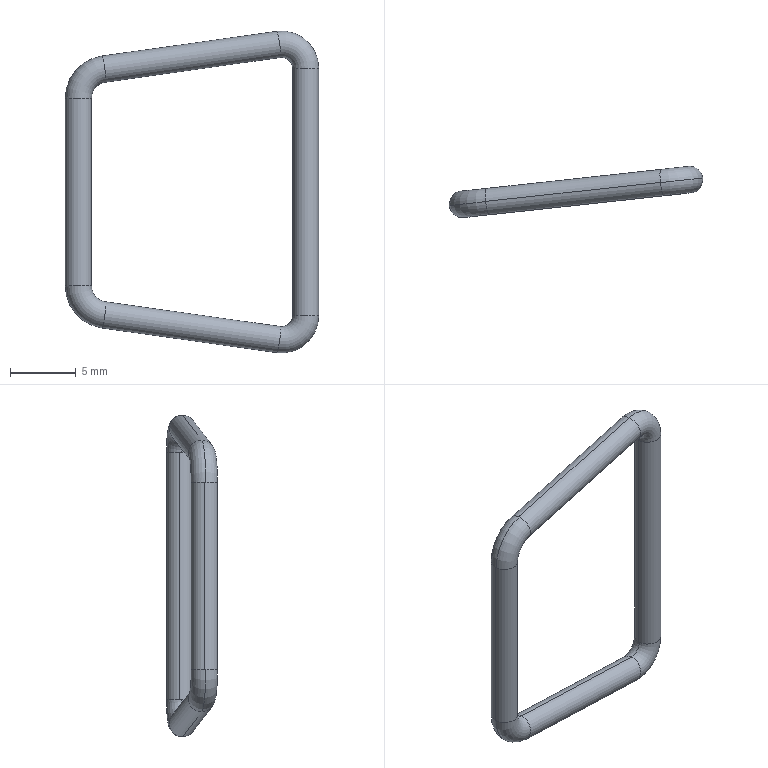Part | SolidWorks | features RefAxis 6, Revolution 4, ICE 3, 3DProfileFeature 2, Extrusion 1 | 1 solid | 16 faces | box 19.288 x 3.878 x 24.478 mm | volume 228.547 mm3 | torus 8 | cylinder 8 | commonest cylinder face diameters 2 x8
STEP:
#1=CARTESIAN_POINT('',(-18.282,-1.986,7.127));
#2=VERTEX_POINT('',#1);
#3=CARTESIAN_POINT('',(-18.288,-1.878,7.127));
#4=VERTEX_POINT('',#3);
#5=CARTESIAN_POINT('',(-17.288,-1.878,7.127));
#6=DIRECTION('',(0.,0.,-1.));
#7=DIRECTION('',(-0.9957,-0.09296,0.));
#8=AXIS2_PLACEMENT_3D('',#5,#6,#7);
#9=CIRCLE('',#8,1.);
#10=EDGE_CURVE('',#2,#4,#9,.T.);
#11=ORIENTED_EDGE('',*,*,#10,.F.);
#12=CARTESIAN_POINT('',(-15.512,-1.685,10.333));
#13=VERTEX_POINT('',#12);
#14=CARTESIAN_POINT('',(-15.064,-1.636,7.127));
#15=DIRECTION('',(-0.108,0.9942,0.));
#16=DIRECTION('',(-0.9942,-0.108,0.));
#17=AXIS2_PLACEMENT_3D('',#14,#15,#16);
#18=CIRCLE('',#17,3.237);
#19=EDGE_CURVE('',#2,#13,#18,.T.);
#20=ORIENTED_EDGE('',*,*,#19,.T.);
#21=CARTESIAN_POINT('',(-15.513,-1.67,10.333));
#22=VERTEX_POINT('',#21);
#23=CARTESIAN_POINT('',(-15.373,-1.67,9.342));
#24=DIRECTION('',(-0.9845,-0.1069,-0.1392));
#25=DIRECTION('',(-0.14,0.,0.9902));
#26=AXIS2_PLACEMENT_3D('',#23,#24,#25);
#27=CIRCLE('',#26,1.);
#28=EDGE_CURVE('',#13,#22,#27,.T.);
#29=ORIENTED_EDGE('',*,*,#28,.T.);
#30=CARTESIAN_POINT('',(-15.235,-1.655,8.352));
#31=VERTEX_POINT('',#30);
#32=CARTESIAN_POINT('',(-15.373,-1.67,9.342));
#33=DIRECTION('',(-0.9845,-0.1069,-0.1392));
#34=DIRECTION('',(-0.14,0.,0.9902));
#35=AXIS2_PLACEMENT_3D('',#32,#33,#34);
#36=CIRCLE('',#35,1.);
#37=EDGE_CURVE('',#22,#31,#36,.T.);
#38=ORIENTED_EDGE('',*,*,#37,.T.);
#39=CARTESIAN_POINT('',(-16.293,-1.77,7.127));
#40=VERTEX_POINT('',#39);
#41=CARTESIAN_POINT('',(-15.064,-1.636,7.127));
#42=DIRECTION('',(-0.108,0.9942,0.));
#43=DIRECTION('',(-0.9942,-0.108,0.));
#44=AXIS2_PLACEMENT_3D('',#41,#42,#43);
#45=CIRCLE('',#44,1.237);
#46=EDGE_CURVE('',#40,#31,#45,.T.);
#47=ORIENTED_EDGE('',*,*,#46,.F.);
#48=CARTESIAN_POINT('',(-17.288,-1.878,7.127));
#49=DIRECTION('',(0.,0.,-1.));
#50=DIRECTION('',(-0.9957,-0.09296,0.));
#51=AXIS2_PLACEMENT_3D('',#48,#49,#50);
#52=CIRCLE('',#51,1.);
#53=EDGE_CURVE('',#4,#40,#52,.T.);
#54=ORIENTED_EDGE('',*,*,#53,.F.);
#55=EDGE_LOOP('',(#11,#20,#29,#38,#47,#54));
#56=FACE_OUTER_BOUND('',#55,.T.);
#57=CARTESIAN_POINT('',(-15.064,-1.636,7.127));
#58=DIRECTION('',(-0.108,0.9942,0.));
#59=DIRECTION('',(-0.9942,-0.108,0.));
#60=AXIS2_PLACEMENT_3D('',#57,#58,#59);
#61=TOROIDAL_SURFACE('',#60,2.237,1.);
#62=ADVANCED_FACE('',(#56),#61,.T.);
#63=CARTESIAN_POINT('',(-18.282,-1.986,-7.127));
#64=VERTEX_POINT('',#63);
#65=CARTESIAN_POINT('',(-16.288,-1.878,-7.127));
#66=VERTEX_POINT('',#65);
#67=CARTESIAN_POINT('',(-17.288,-1.878,-7.127));
#68=DIRECTION('',(0.,0.,1.));
#69=DIRECTION('',(0.9957,0.09296,0.));
#70=AXIS2_PLACEMENT_3D('',#67,#68,#69);
#71=CIRCLE('',#70,1.);
#72=EDGE_CURVE('',#64,#66,#71,.T.);
#73=ORIENTED_EDGE('',*,*,#72,.F.);
#74=CARTESIAN_POINT('',(-15.512,-1.685,-10.333));
#75=VERTEX_POINT('',#74);
#76=CARTESIAN_POINT('',(-15.064,-1.636,-7.127));
#77=DIRECTION('',(0.108,-0.9942,0.));
#78=DIRECTION('',(0.9942,0.108,0.));
#79=AXIS2_PLACEMENT_3D('',#76,#77,#78);
#80=CIRCLE('',#79,3.237);
#81=EDGE_CURVE('',#64,#75,#80,.T.);
#82=ORIENTED_EDGE('',*,*,#81,.T.);
#83=CARTESIAN_POINT('',(-15.233,-1.67,-8.352));
#84=VERTEX_POINT('',#83);
#85=CARTESIAN_POINT('',(-15.373,-1.67,-9.342));
#86=DIRECTION('',(-0.9845,-0.1069,0.1392));
#87=DIRECTION('',(0.14,0.,0.9902));
#88=AXIS2_PLACEMENT_3D('',#85,#86,#87);
#89=CIRCLE('',#88,1.);
#90=EDGE_CURVE('',#75,#84,#89,.T.);
#91=ORIENTED_EDGE('',*,*,#90,.T.);
#92=CARTESIAN_POINT('',(-15.235,-1.655,-8.352));
#93=VERTEX_POINT('',#92);
#94=CARTESIAN_POINT('',(-15.373,-1.67,-9.342));
#95=DIRECTION('',(-0.9845,-0.1069,0.1392));
#96=DIRECTION('',(0.14,0.,0.9902));
#97=AXIS2_PLACEMENT_3D('',#94,#95,#96);
#98=CIRCLE('',#97,1.);
#99=EDGE_CURVE('',#84,#93,#98,.T.);
#100=ORIENTED_EDGE('',*,*,#99,.T.);
#101=CARTESIAN_POINT('',(-16.293,-1.77,-7.127));
#102=VERTEX_POINT('',#101);
#103=CARTESIAN_POINT('',(-15.064,-1.636,-7.127));
#104=DIRECTION('',(0.108,-0.9942,0.));
#105=DIRECTION('',(0.9942,0.108,0.));
#106=AXIS2_PLACEMENT_3D('',#103,#104,#105);
#107=CIRCLE('',#106,1.237);
#108=EDGE_CURVE('',#102,#93,#107,.T.);
#109=ORIENTED_EDGE('',*,*,#108,.F.);
#110=CARTESIAN_POINT('',(-17.288,-1.878,-7.127));
#111=DIRECTION('',(0.,0.,1.));
#112=DIRECTION('',(0.9957,0.09296,0.));
#113=AXIS2_PLACEMENT_3D('',#110,#111,#112);
#114=CIRCLE('',#113,1.);
#115=EDGE_CURVE('',#66,#102,#114,.T.);
#116=ORIENTED_EDGE('',*,*,#115,.F.);
#117=EDGE_LOOP('',(#73,#82,#91,#100,#109,#116));
#118=FACE_OUTER_BOUND('',#117,.T.);
#119=CARTESIAN_POINT('',(-15.064,-1.636,-7.127));
#120=DIRECTION('',(0.108,-0.9942,0.));
#121=DIRECTION('',(0.9942,0.108,0.));
#122=AXIS2_PLACEMENT_3D('',#119,#120,#121);
#123=TOROIDAL_SURFACE('',#122,2.237,1.);
#124=ADVANCED_FACE('',(#118),#123,.T.);
#125=CARTESIAN_POINT('',(-2.221,-0.2413,12.212));
#126=VERTEX_POINT('',#125);
#127=CARTESIAN_POINT('',(-2.223,-0.2263,12.211));
#128=VERTEX_POINT('',#127);
#129=CARTESIAN_POINT('',(-2.083,-0.2263,11.221));
#130=DIRECTION('',(-0.9845,-0.1069,-0.1392));
#131=DIRECTION('',(-0.1259,-0.1223,0.9845));
#132=AXIS2_PLACEMENT_3D('',#129,#130,#131);
#133=CIRCLE('',#132,1.);
#134=EDGE_CURVE('',#126,#128,#133,.T.);
#135=ORIENTED_EDGE('',*,*,#134,.F.);
#136=CARTESIAN_POINT('',(0.9942,0.108,9.4));
#137=VERTEX_POINT('',#136);
#138=CARTESIAN_POINT('',(-1.828,-0.1986,9.4));
#139=DIRECTION('',(-0.108,0.9942,0.));
#140=DIRECTION('',(-0.9942,-0.108,0.));
#141=AXIS2_PLACEMENT_3D('',#138,#139,#140);
#142=CIRCLE('',#141,2.839);
#143=EDGE_CURVE('',#126,#137,#142,.T.);
#144=ORIENTED_EDGE('',*,*,#143,.T.);
#145=CARTESIAN_POINT('',(-1.,0.,9.4));
#146=VERTEX_POINT('',#145);
#147=CARTESIAN_POINT('',(0.,0.,9.4));
#148=DIRECTION('',(0.,0.,1.));
#149=DIRECTION('',(1.,0.,0.));
#150=AXIS2_PLACEMENT_3D('',#147,#148,#149);
#151=CIRCLE('',#150,1.);
#152=EDGE_CURVE('',#137,#146,#151,.T.);
#153=ORIENTED_EDGE('',*,*,#152,.T.);
#154=CARTESIAN_POINT('',(-0.9942,-0.108,9.4));
#155=VERTEX_POINT('',#154);
#156=CARTESIAN_POINT('',(0.,0.,9.4));
#157=DIRECTION('',(0.,0.,1.));
#158=DIRECTION('',(1.,0.,0.));
#159=AXIS2_PLACEMENT_3D('',#156,#157,#158);
#160=CIRCLE('',#159,1.);
#161=EDGE_CURVE('',#146,#155,#160,.T.);
#162=ORIENTED_EDGE('',*,*,#161,.T.);
#163=CARTESIAN_POINT('',(-1.945,-0.2112,10.231));
#164=VERTEX_POINT('',#163);
#165=CARTESIAN_POINT('',(-1.828,-0.1986,9.4));
#166=DIRECTION('',(-0.108,0.9942,0.));
#167=DIRECTION('',(-0.9942,-0.108,0.));
#168=AXIS2_PLACEMENT_3D('',#165,#166,#167);
#169=CIRCLE('',#168,0.8392);
#170=EDGE_CURVE('',#164,#155,#169,.T.);
#171=ORIENTED_EDGE('',*,*,#170,.F.);
#172=CARTESIAN_POINT('',(-2.083,-0.2263,11.221));
#173=DIRECTION('',(-0.9845,-0.1069,-0.1392));
#174=DIRECTION('',(-0.1259,-0.1223,0.9845));
#175=AXIS2_PLACEMENT_3D('',#172,#173,#174);
#176=CIRCLE('',#175,1.);
#177=EDGE_CURVE('',#128,#164,#176,.T.);
#178=ORIENTED_EDGE('',*,*,#177,.F.);
#179=EDGE_LOOP('',(#135,#144,#153,#162,#171,#178));
#180=FACE_OUTER_BOUND('',#179,.T.);
#181=CARTESIAN_POINT('',(-1.828,-0.1986,9.4));
#182=DIRECTION('',(-0.108,0.9942,0.));
#183=DIRECTION('',(-0.9942,-0.108,0.));
#184=AXIS2_PLACEMENT_3D('',#181,#182,#183);
#185=TOROIDAL_SURFACE('',#184,1.839,1.);
#186=ADVANCED_FACE('',(#180),#185,.T.);
#187=CARTESIAN_POINT('',(-1.943,-0.2263,-10.231));
#188=VERTEX_POINT('',#187);
#189=CARTESIAN_POINT('',(-2.221,-0.2413,-12.212));
#190=VERTEX_POINT('',#189);
#191=CARTESIAN_POINT('',(-2.083,-0.2263,-11.221));
#192=DIRECTION('',(0.9845,0.1069,-0.1392));
#193=DIRECTION('',(-0.1259,-0.1223,-0.9845));
#194=AXIS2_PLACEMENT_3D('',#191,#192,#193);
#195=CIRCLE('',#194,1.);
#196=EDGE_CURVE('',#188,#190,#195,.T.);
#197=ORIENTED_EDGE('',*,*,#196,.T.);
#198=CARTESIAN_POINT('',(0.9942,0.108,-9.4));
#199=VERTEX_POINT('',#198);
#200=CARTESIAN_POINT('',(-1.828,-0.1986,-9.4));
#201=DIRECTION('',(0.108,-0.9942,0.));
#202=DIRECTION('',(0.9942,0.108,0.));
#203=AXIS2_PLACEMENT_3D('',#200,#201,#202);
#204=CIRCLE('',#203,2.839);
#205=EDGE_CURVE('',#190,#199,#204,.T.);
#206=ORIENTED_EDGE('',*,*,#205,.T.);
#207=CARTESIAN_POINT('',(1.,0.,-9.4));
#208=VERTEX_POINT('',#207);
#209=CARTESIAN_POINT('',(0.,0.,-9.4));
#210=DIRECTION('',(0.,0.,1.));
#211=DIRECTION('',(1.,0.,0.));
#212=AXIS2_PLACEMENT_3D('',#209,#210,#211);
#213=CIRCLE('',#212,1.);
#214=EDGE_CURVE('',#208,#199,#213,.T.);
#215=ORIENTED_EDGE('',*,*,#214,.F.);
#216=CARTESIAN_POINT('',(-0.9942,-0.108,-9.4));
#217=VERTEX_POINT('',#216);
#218=CARTESIAN_POINT('',(0.,0.,-9.4));
#219=DIRECTION('',(0.,0.,1.));
#220=DIRECTION('',(1.,0.,0.));
#221=AXIS2_PLACEMENT_3D('',#218,#219,#220);
#222=CIRCLE('',#221,1.);
#223=EDGE_CURVE('',#217,#208,#222,.T.);
#224=ORIENTED_EDGE('',*,*,#223,.F.);
#225=CARTESIAN_POINT('',(-1.945,-0.2112,-10.231));
#226=VERTEX_POINT('',#225);
#227=CARTESIAN_POINT('',(-1.828,-0.1986,-9.4));
#228=DIRECTION('',(0.108,-0.9942,0.));
#229=DIRECTION('',(0.9942,0.108,0.));
#230=AXIS2_PLACEMENT_3D('',#227,#228,#229);
#231=CIRCLE('',#230,0.8392);
#232=EDGE_CURVE('',#226,#217,#231,.T.);
#233=ORIENTED_EDGE('',*,*,#232,.F.);
#234=CARTESIAN_POINT('',(-2.083,-0.2263,-11.221));
#235=DIRECTION('',(0.9845,0.1069,-0.1392));
#236=DIRECTION('',(-0.1259,-0.1223,-0.9845));
#237=AXIS2_PLACEMENT_3D('',#234,#235,#236);
#238=CIRCLE('',#237,1.);
#239=EDGE_CURVE('',#226,#188,#238,.T.);
#240=ORIENTED_EDGE('',*,*,#239,.T.);
#241=EDGE_LOOP('',(#197,#206,#215,#224,#233,#240));
#242=FACE_OUTER_BOUND('',#241,.T.);
#243=CARTESIAN_POINT('',(-1.828,-0.1986,-9.4));
#244=DIRECTION('',(0.108,-0.9942,0.));
#245=DIRECTION('',(0.9942,0.108,0.));
#246=AXIS2_PLACEMENT_3D('',#243,#244,#245);
#247=TOROIDAL_SURFACE('',#246,1.839,1.);
#248=ADVANCED_FACE('',(#242),#247,.T.);
#249=ORIENTED_EDGE('',*,*,#53,.T.);
#250=CARTESIAN_POINT('',(-16.288,-1.878,7.127));
#251=VERTEX_POINT('',#250);
#252=CARTESIAN_POINT('',(-17.288,-1.878,7.127));
#253=DIRECTION('',(0.,0.,-1.));
#254=DIRECTION('',(-0.9957,-0.09296,0.));
#255=AXIS2_PLACEMENT_3D('',#252,#253,#254);
#256=CIRCLE('',#255,1.);
#257=EDGE_CURVE('',#40,#251,#256,.T.);
#258=ORIENTED_EDGE('',*,*,#257,.T.);
#259=CARTESIAN_POINT('',(-16.288,-1.878,7.128));
#260=DIRECTION('',(0.,0.,-1.));
#261=VECTOR('',#260,1000.);
#262=LINE('',#259,#261);
#263=EDGE_CURVE('',#251,#66,#262,.T.);
#264=ORIENTED_EDGE('',*,*,#263,.T.);
#265=ORIENTED_EDGE('',*,*,#115,.T.);
#266=CARTESIAN_POINT('',(-18.288,-1.878,-7.127));
#267=VERTEX_POINT('',#266);
#268=CARTESIAN_POINT('',(-17.288,-1.878,-7.127));
#269=DIRECTION('',(0.,0.,1.));
#270=DIRECTION('',(0.9957,0.09296,0.));
#271=AXIS2_PLACEMENT_3D('',#268,#269,#270);
#272=CIRCLE('',#271,1.);
#273=EDGE_CURVE('',#102,#267,#272,.T.);
#274=ORIENTED_EDGE('',*,*,#273,.T.);
#275=CARTESIAN_POINT('',(-18.288,-1.878,7.128));
#276=DIRECTION('',(0.,0.,-1.));
#277=VECTOR('',#276,1000.);
#278=LINE('',#275,#277);
#279=EDGE_CURVE('',#4,#267,#278,.T.);
#280=ORIENTED_EDGE('',*,*,#279,.F.);
#281=EDGE_LOOP('',(#249,#258,#264,#265,#274,#280));
#282=FACE_OUTER_BOUND('',#281,.T.);
#283=CARTESIAN_POINT('',(-17.288,-1.878,7.128));
#284=DIRECTION('',(0.,0.,-1.));
#285=DIRECTION('',(-1.,0.,0.));
#286=AXIS2_PLACEMENT_3D('',#283,#284,#285);
#287=CYLINDRICAL_SURFACE('',#286,1.);
#288=ADVANCED_FACE('',(#282),#287,.T.);
#289=ORIENTED_EDGE('',*,*,#37,.F.);
#290=CARTESIAN_POINT('',(-15.513,-1.67,10.333));
#291=DIRECTION('',(0.9845,0.1069,0.1392));
#292=VECTOR('',#291,1000.);
#293=LINE('',#290,#292);
#294=EDGE_CURVE('',#22,#128,#293,.T.);
#295=ORIENTED_EDGE('',*,*,#294,.T.);
#296=ORIENTED_EDGE('',*,*,#177,.T.);
#297=CARTESIAN_POINT('',(-1.943,-0.2263,10.231));
#298=VERTEX_POINT('',#297);
#299=CARTESIAN_POINT('',(-2.083,-0.2263,11.221));
#300=DIRECTION('',(-0.9845,-0.1069,-0.1392));
#301=DIRECTION('',(-0.1259,-0.1223,0.9845));
#302=AXIS2_PLACEMENT_3D('',#299,#300,#301);
#303=CIRCLE('',#302,1.);
#304=EDGE_CURVE('',#164,#298,#303,.T.);
#305=ORIENTED_EDGE('',*,*,#304,.T.);
#306=CARTESIAN_POINT('',(-15.233,-1.67,8.352));
#307=VERTEX_POINT('',#306);
#308=CARTESIAN_POINT('',(-15.233,-1.67,8.352));
#309=DIRECTION('',(0.9845,0.1069,0.1392));
#310=VECTOR('',#309,1000.);
#311=LINE('',#308,#310);
#312=EDGE_CURVE('',#307,#298,#311,.T.);
#313=ORIENTED_EDGE('',*,*,#312,.F.);
#314=CARTESIAN_POINT('',(-15.373,-1.67,9.342));
#315=DIRECTION('',(-0.9845,-0.1069,-0.1392));
#316=DIRECTION('',(-0.14,0.,0.9902));
#317=AXIS2_PLACEMENT_3D('',#314,#315,#316);
#318=CIRCLE('',#317,1.);
#319=EDGE_CURVE('',#31,#307,#318,.T.);
#320=ORIENTED_EDGE('',*,*,#319,.F.);
#321=EDGE_LOOP('',(#289,#295,#296,#305,#313,#320));
#322=FACE_OUTER_BOUND('',#321,.T.);
#323=CARTESIAN_POINT('',(-15.373,-1.67,9.342));
#324=DIRECTION('',(0.9845,0.1069,0.1392));
#325=DIRECTION('',(0.14,0.,-0.9902));
#326=AXIS2_PLACEMENT_3D('',#323,#324,#325);
#327=CYLINDRICAL_SURFACE('',#326,1.);
#328=ADVANCED_FACE('',(#322),#327,.T.);
#329=ORIENTED_EDGE('',*,*,#99,.F.);
#330=CARTESIAN_POINT('',(-15.233,-1.67,-8.352));
#331=DIRECTION('',(0.9845,0.1069,-0.1392));
#332=VECTOR('',#331,1000.);
#333=LINE('',#330,#332);
#334=EDGE_CURVE('',#84,#188,#333,.T.);
#335=ORIENTED_EDGE('',*,*,#334,.T.);
#336=ORIENTED_EDGE('',*,*,#239,.F.);
#337=CARTESIAN_POINT('',(-2.223,-0.2263,-12.211));
#338=VERTEX_POINT('',#337);
#339=CARTESIAN_POINT('',(-2.083,-0.2263,-11.221));
#340=DIRECTION('',(0.9845,0.1069,-0.1392));
#341=DIRECTION('',(-0.1259,-0.1223,-0.9845));
#342=AXIS2_PLACEMENT_3D('',#339,#340,#341);
#343=CIRCLE('',#342,1.);
#344=EDGE_CURVE('',#338,#226,#343,.T.);
#345=ORIENTED_EDGE('',*,*,#344,.F.);
#346=CARTESIAN_POINT('',(-15.513,-1.67,-10.333));
#347=VERTEX_POINT('',#346);
#348=CARTESIAN_POINT('',(-15.513,-1.67,-10.333));
#349=DIRECTION('',(0.9845,0.1069,-0.1392));
#350=VECTOR('',#349,1000.);
#351=LINE('',#348,#350);
#352=EDGE_CURVE('',#347,#338,#351,.T.);
#353=ORIENTED_EDGE('',*,*,#352,.F.);
#354=CARTESIAN_POINT('',(-15.373,-1.67,-9.342));
#355=DIRECTION('',(-0.9845,-0.1069,0.1392));
#356=DIRECTION('',(0.14,0.,0.9902));
#357=AXIS2_PLACEMENT_3D('',#354,#355,#356);
#358=CIRCLE('',#357,1.);
#359=EDGE_CURVE('',#93,#347,#358,.T.);
#360=ORIENTED_EDGE('',*,*,#359,.F.);
#361=EDGE_LOOP('',(#329,#335,#336,#345,#353,#360));
#362=FACE_OUTER_BOUND('',#361,.T.);
#363=CARTESIAN_POINT('',(-15.373,-1.67,-9.342));
#364=DIRECTION('',(0.9845,0.1069,-0.1392));
#365=DIRECTION('',(-0.14,0.,-0.9902));
#366=AXIS2_PLACEMENT_3D('',#363,#364,#365);
#367=CYLINDRICAL_SURFACE('',#366,1.);
#368=ADVANCED_FACE('',(#362),#367,.T.);
#369=CARTESIAN_POINT('',(1.,0.,9.4));
#370=VERTEX_POINT('',#369);
#371=CARTESIAN_POINT('',(0.,0.,9.4));
#372=DIRECTION('',(0.,0.,1.));
#373=DIRECTION('',(1.,0.,0.));
#374=AXIS2_PLACEMENT_3D('',#371,#372,#373);
#375=CIRCLE('',#374,1.);
#376=EDGE_CURVE('',#370,#137,#375,.T.);
#377=ORIENTED_EDGE('',*,*,#376,.F.);
#378=CARTESIAN_POINT('',(1.,0.,9.4));
#379=DIRECTION('',(0.,0.,-1.));
#380=VECTOR('',#379,1000.);
#381=LINE('',#378,#380);
#382=EDGE_CURVE('',#370,#208,#381,.T.);
#383=ORIENTED_EDGE('',*,*,#382,.T.);
#384=ORIENTED_EDGE('',*,*,#214,.T.);
#385=CARTESIAN_POINT('',(-1.,0.,-9.4));
#386=VERTEX_POINT('',#385);
#387=CARTESIAN_POINT('',(0.,0.,-9.4));
#388=DIRECTION('',(0.,0.,1.));
#389=DIRECTION('',(1.,0.,0.));
#390=AXIS2_PLACEMENT_3D('',#387,#388,#389);
#391=CIRCLE('',#390,1.);
#392=EDGE_CURVE('',#199,#386,#391,.T.);
#393=ORIENTED_EDGE('',*,*,#392,.T.);
#394=CARTESIAN_POINT('',(-1.,0.,9.4));
#395=DIRECTION('',(0.,0.,-1.));
#396=VECTOR('',#395,1000.);
#397=LINE('',#394,#396);
#398=EDGE_CURVE('',#146,#386,#397,.T.);
#399=ORIENTED_EDGE('',*,*,#398,.F.);
#400=ORIENTED_EDGE('',*,*,#152,.F.);
#401=EDGE_LOOP('',(#377,#383,#384,#393,#399,#400));
#402=FACE_OUTER_BOUND('',#401,.T.);
#403=CARTESIAN_POINT('',(0.,0.,9.4));
#404=DIRECTION('',(0.,0.,-1.));
#405=DIRECTION('',(-1.,0.,0.));
#406=AXIS2_PLACEMENT_3D('',#403,#404,#405);
#407=CYLINDRICAL_SURFACE('',#406,1.);
#408=ADVANCED_FACE('',(#402),#407,.T.);
#409=ORIENTED_EDGE('',*,*,#382,.F.);
#410=CARTESIAN_POINT('',(0.,0.,9.4));
#411=DIRECTION('',(0.,0.,1.));
#412=DIRECTION('',(1.,0.,0.));
#413=AXIS2_PLACEMENT_3D('',#410,#411,#412);
#414=CIRCLE('',#413,1.);
#415=EDGE_CURVE('',#155,#370,#414,.T.);
#416=ORIENTED_EDGE('',*,*,#415,.F.);
#417=ORIENTED_EDGE('',*,*,#161,.F.);
#418=ORIENTED_EDGE('',*,*,#398,.T.);
#419=CARTESIAN_POINT('',(0.,0.,-9.4));
#420=DIRECTION('',(0.,0.,1.));
#421=DIRECTION('',(1.,0.,0.));
#422=AXIS2_PLACEMENT_3D('',#419,#420,#421);
#423=CIRCLE('',#422,1.);
#424=EDGE_CURVE('',#386,#217,#423,.T.);
#425=ORIENTED_EDGE('',*,*,#424,.T.);
#426=ORIENTED_EDGE('',*,*,#223,.T.);
#427=EDGE_LOOP('',(#409,#416,#417,#418,#425,#426));
#428=FACE_OUTER_BOUND('',#427,.T.);
#429=CARTESIAN_POINT('',(0.,0.,9.4));
#430=DIRECTION('',(0.,0.,-1.));
#431=DIRECTION('',(-1.,0.,0.));
#432=AXIS2_PLACEMENT_3D('',#429,#430,#431);
#433=CYLINDRICAL_SURFACE('',#432,1.);
#434=ADVANCED_FACE('',(#428),#433,.T.);
#435=ORIENTED_EDGE('',*,*,#205,.F.);
#436=CARTESIAN_POINT('',(-2.083,-0.2263,-11.221));
#437=DIRECTION('',(0.9845,0.1069,-0.1392));
#438=DIRECTION('',(-0.1259,-0.1223,-0.9845));
#439=AXIS2_PLACEMENT_3D('',#436,#437,#438);
#440=CIRCLE('',#439,1.);
#441=EDGE_CURVE('',#190,#338,#440,.T.);
#442=ORIENTED_EDGE('',*,*,#441,.T.);
#443=ORIENTED_EDGE('',*,*,#344,.T.);
#444=ORIENTED_EDGE('',*,*,#232,.T.);
#445=ORIENTED_EDGE('',*,*,#424,.F.);
#446=ORIENTED_EDGE('',*,*,#392,.F.);
#447=EDGE_LOOP('',(#435,#442,#443,#444,#445,#446));
#448=FACE_OUTER_BOUND('',#447,.T.);
#449=CARTESIAN_POINT('',(-1.828,-0.1986,-9.4));
#450=DIRECTION('',(0.108,-0.9942,0.));
#451=DIRECTION('',(0.9942,0.108,0.));
#452=AXIS2_PLACEMENT_3D('',#449,#450,#451);
#453=TOROIDAL_SURFACE('',#452,1.839,1.);
#454=ADVANCED_FACE('',(#448),#453,.T.);
#455=ORIENTED_EDGE('',*,*,#334,.F.);
#456=ORIENTED_EDGE('',*,*,#90,.F.);
#457=CARTESIAN_POINT('',(-15.373,-1.67,-9.342));
#458=DIRECTION('',(-0.9845,-0.1069,0.1392));
#459=DIRECTION('',(0.14,0.,0.9902));
#460=AXIS2_PLACEMENT_3D('',#457,#458,#459);
#461=CIRCLE('',#460,1.);
#462=EDGE_CURVE('',#347,#75,#461,.T.);
#463=ORIENTED_EDGE('',*,*,#462,.F.);
#464=ORIENTED_EDGE('',*,*,#352,.T.);
#465=ORIENTED_EDGE('',*,*,#441,.F.);
#466=ORIENTED_EDGE('',*,*,#196,.F.);
#467=EDGE_LOOP('',(#455,#456,#463,#464,#465,#466));
#468=FACE_OUTER_BOUND('',#467,.T.);
#469=CARTESIAN_POINT('',(-15.373,-1.67,-9.342));
#470=DIRECTION('',(0.9845,0.1069,-0.1392));
#471=DIRECTION('',(-0.14,0.,-0.9902));
#472=AXIS2_PLACEMENT_3D('',#469,#470,#471);
#473=CYLINDRICAL_SURFACE('',#472,1.);
#474=ADVANCED_FACE('',(#468),#473,.T.);
#475=ORIENTED_EDGE('',*,*,#143,.F.);
#476=CARTESIAN_POINT('',(-2.083,-0.2263,11.221));
#477=DIRECTION('',(-0.9845,-0.1069,-0.1392));
#478=DIRECTION('',(-0.1259,-0.1223,0.9845));
#479=AXIS2_PLACEMENT_3D('',#476,#477,#478);
#480=CIRCLE('',#479,1.);
#481=EDGE_CURVE('',#298,#126,#480,.T.);
#482=ORIENTED_EDGE('',*,*,#481,.F.);
#483=ORIENTED_EDGE('',*,*,#304,.F.);
#484=ORIENTED_EDGE('',*,*,#170,.T.);
#485=ORIENTED_EDGE('',*,*,#415,.T.);
#486=ORIENTED_EDGE('',*,*,#376,.T.);
#487=EDGE_LOOP('',(#475,#482,#483,#484,#485,#486));
#488=FACE_OUTER_BOUND('',#487,.T.);
#489=CARTESIAN_POINT('',(-1.828,-0.1986,9.4));
#490=DIRECTION('',(-0.108,0.9942,0.));
#491=DIRECTION('',(-0.9942,-0.108,0.));
#492=AXIS2_PLACEMENT_3D('',#489,#490,#491);
#493=TOROIDAL_SURFACE('',#492,1.839,1.);
#494=ADVANCED_FACE('',(#488),#493,.T.);
#495=ORIENTED_EDGE('',*,*,#294,.F.);
#496=ORIENTED_EDGE('',*,*,#28,.F.);
#497=CARTESIAN_POINT('',(-15.373,-1.67,9.342));
#498=DIRECTION('',(-0.9845,-0.1069,-0.1392));
#499=DIRECTION('',(-0.14,0.,0.9902));
#500=AXIS2_PLACEMENT_3D('',#497,#498,#499);
#501=CIRCLE('',#500,1.);
#502=EDGE_CURVE('',#307,#13,#501,.T.);
#503=ORIENTED_EDGE('',*,*,#502,.F.);
#504=ORIENTED_EDGE('',*,*,#312,.T.);
#505=ORIENTED_EDGE('',*,*,#481,.T.);
#506=ORIENTED_EDGE('',*,*,#134,.T.);
#507=EDGE_LOOP('',(#495,#496,#503,#504,#505,#506));
#508=FACE_OUTER_BOUND('',#507,.T.);
#509=CARTESIAN_POINT('',(-15.373,-1.67,9.342));
#510=DIRECTION('',(0.9845,0.1069,0.1392));
#511=DIRECTION('',(0.14,0.,-0.9902));
#512=AXIS2_PLACEMENT_3D('',#509,#510,#511);
#513=CYLINDRICAL_SURFACE('',#512,1.);
#514=ADVANCED_FACE('',(#508),#513,.T.);
#515=ORIENTED_EDGE('',*,*,#81,.F.);
#516=CARTESIAN_POINT('',(-17.288,-1.878,-7.127));
#517=DIRECTION('',(0.,0.,1.));
#518=DIRECTION('',(0.9957,0.09296,0.));
#519=AXIS2_PLACEMENT_3D('',#516,#517,#518);
#520=CIRCLE('',#519,1.);
#521=EDGE_CURVE('',#267,#64,#520,.T.);
#522=ORIENTED_EDGE('',*,*,#521,.F.);
#523=ORIENTED_EDGE('',*,*,#273,.F.);
#524=ORIENTED_EDGE('',*,*,#108,.T.);
#525=ORIENTED_EDGE('',*,*,#359,.T.);
#526=ORIENTED_EDGE('',*,*,#462,.T.);
#527=EDGE_LOOP('',(#515,#522,#523,#524,#525,#526));
#528=FACE_OUTER_BOUND('',#527,.T.);
#529=CARTESIAN_POINT('',(-15.064,-1.636,-7.127));
#530=DIRECTION('',(0.108,-0.9942,0.));
#531=DIRECTION('',(0.9942,0.108,0.));
#532=AXIS2_PLACEMENT_3D('',#529,#530,#531);
#533=TOROIDAL_SURFACE('',#532,2.237,1.);
#534=ADVANCED_FACE('',(#528),#533,.T.);
#535=ORIENTED_EDGE('',*,*,#19,.F.);
#536=CARTESIAN_POINT('',(-17.288,-1.878,7.127));
#537=DIRECTION('',(0.,0.,-1.));
#538=DIRECTION('',(-0.9957,-0.09296,0.));
#539=AXIS2_PLACEMENT_3D('',#536,#537,#538);
#540=CIRCLE('',#539,1.);
#541=EDGE_CURVE('',#251,#2,#540,.T.);
#542=ORIENTED_EDGE('',*,*,#541,.F.);
#543=ORIENTED_EDGE('',*,*,#257,.F.);
#544=ORIENTED_EDGE('',*,*,#46,.T.);
#545=ORIENTED_EDGE('',*,*,#319,.T.);
#546=ORIENTED_EDGE('',*,*,#502,.T.);
#547=EDGE_LOOP('',(#535,#542,#543,#544,#545,#546));
#548=FACE_OUTER_BOUND('',#547,.T.);
#549=CARTESIAN_POINT('',(-15.064,-1.636,7.127));
#550=DIRECTION('',(-0.108,0.9942,0.));
#551=DIRECTION('',(-0.9942,-0.108,0.));
#552=AXIS2_PLACEMENT_3D('',#549,#550,#551);
#553=TOROIDAL_SURFACE('',#552,2.237,1.);
#554=ADVANCED_FACE('',(#548),#553,.T.);
#555=ORIENTED_EDGE('',*,*,#263,.F.);
#556=ORIENTED_EDGE('',*,*,#541,.T.);
#557=ORIENTED_EDGE('',*,*,#10,.T.);
#558=ORIENTED_EDGE('',*,*,#279,.T.);
#559=ORIENTED_EDGE('',*,*,#521,.T.);
#560=ORIENTED_EDGE('',*,*,#72,.T.);
#561=EDGE_LOOP('',(#555,#556,#557,#558,#559,#560));
#562=FACE_OUTER_BOUND('',#561,.T.);
#563=CARTESIAN_POINT('',(-17.288,-1.878,7.128));
#564=DIRECTION('',(0.,0.,-1.));
#565=DIRECTION('',(-1.,0.,0.));
#566=AXIS2_PLACEMENT_3D('',#563,#564,#565);
#567=CYLINDRICAL_SURFACE('',#566,1.);
#568=ADVANCED_FACE('',(#562),#567,.T.);
#569=CLOSED_SHELL('',(#62,#124,#186,#248,#288,#328,#368,#408,#434,#454,#474,#494,#514,#534,#554,#568));
#570=MANIFOLD_SOLID_BREP('',#569);
#571=CARTESIAN_POINT('',(0.,0.,0.));
#572=DIRECTION('',(0.,0.,1.));
#573=DIRECTION('',(1.,0.,0.));
#574=AXIS2_PLACEMENT_3D('',#571,#572,#573);
#575=(LENGTH_UNIT()NAMED_UNIT(*)SI_UNIT(.MILLI.,.METRE.));
#576=UNCERTAINTY_MEASURE_WITH_UNIT(LENGTH_MEASURE(0.00001),#575,'','');
#577=(NAMED_UNIT(*)PLANE_ANGLE_UNIT()SI_UNIT($,.RADIAN.));
#578=(NAMED_UNIT(*)SI_UNIT($,.STERADIAN.)SOLID_ANGLE_UNIT());
#579=(GEOMETRIC_REPRESENTATION_CONTEXT(3)GLOBAL_UNCERTAINTY_ASSIGNED_CONTEXT((#576))GLOBAL_UNIT_ASSIGNED_CONTEXT((#575,#577,#578))REPRESENTATION_CONTEXT('',''));
#580=ADVANCED_BREP_SHAPE_REPRESENTATION('',(#570,#574),#579);